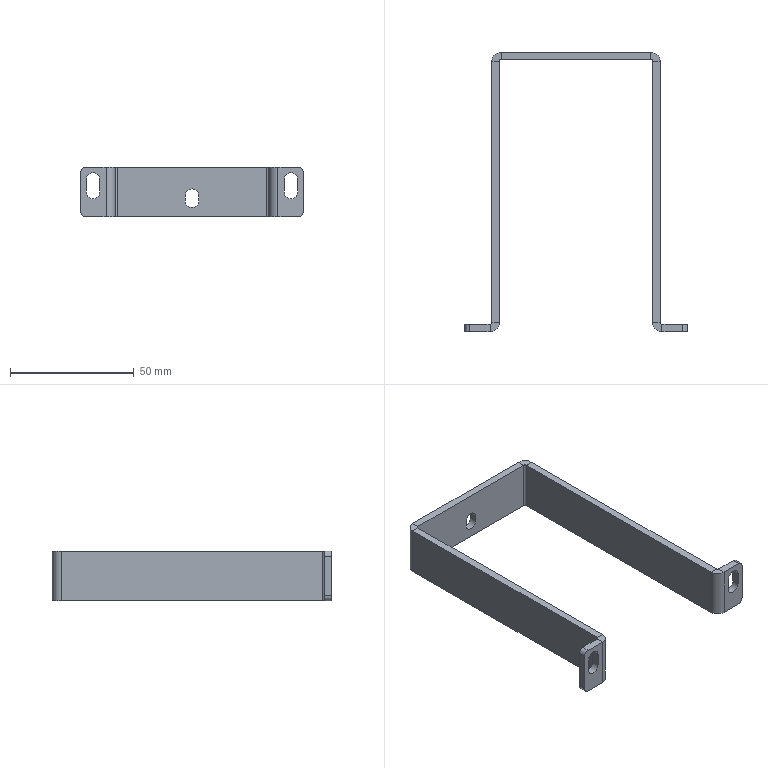Part | STEP file | 1 solid | 57 faces | box 90 x 113 x 20 mm | volume 17947 mm3 | plane 36 | cylinder 21 | commonest cylinder face diameters 5.5 x9 1.473 x4 4 x4 7.473 x4